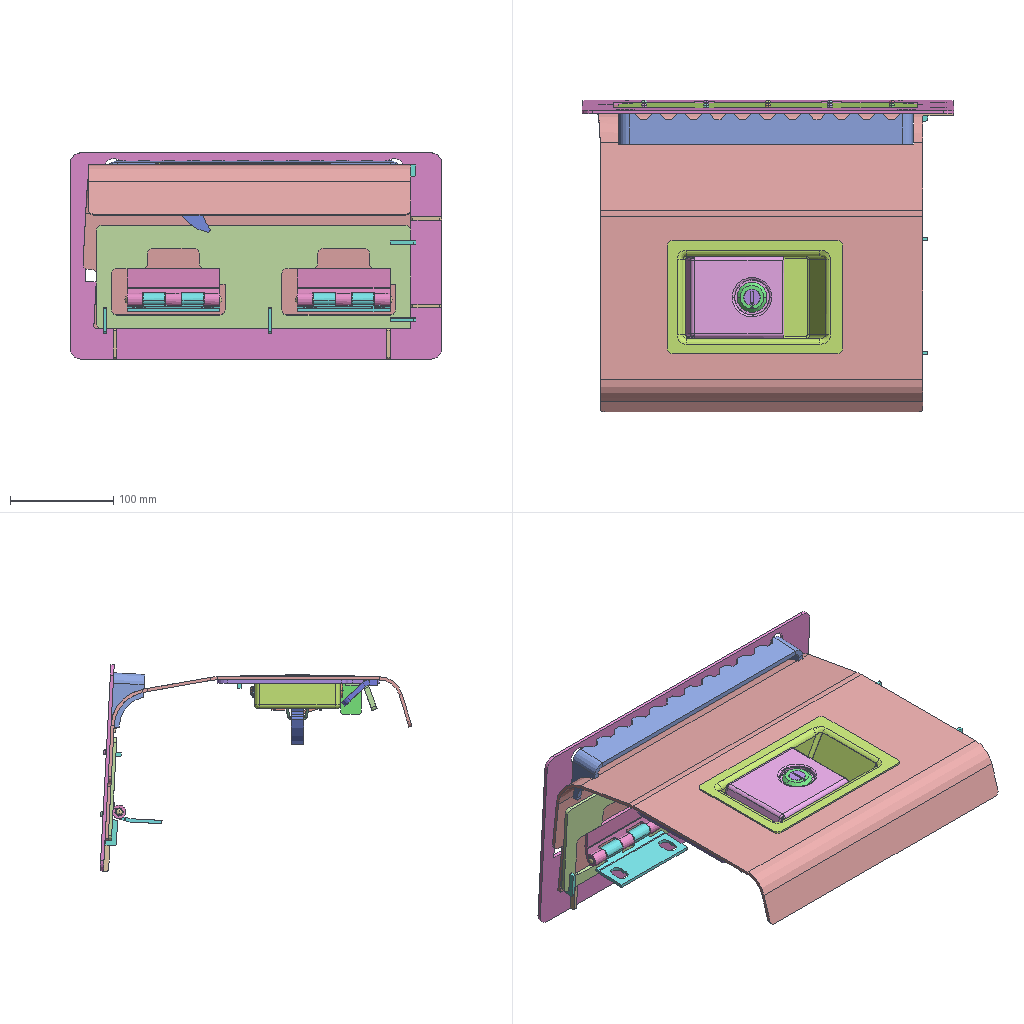Assembly | SolidWorks | 14 different items | 24 placed | box 360 x 302 x 200 mm
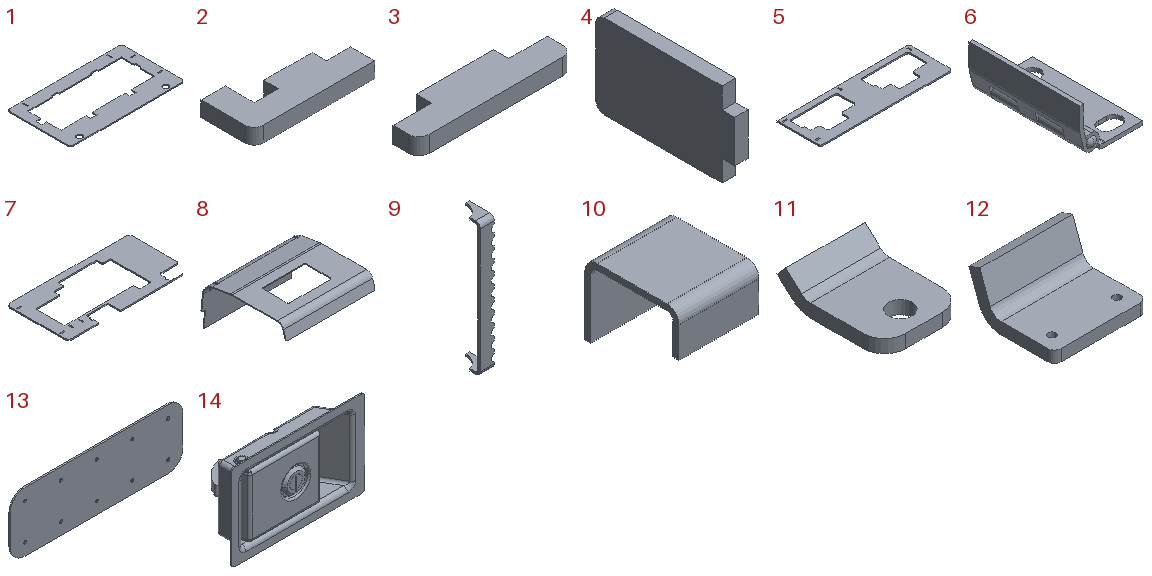Parts list (item | quantity | size | volume | features):
1 | x1 | 360 x 200 x 3.2 mm | 125012 mm3 | features FlatPattern 1, SMBaseFlange 1, SheetMetal 1
2 | x6 | 25 x 11 x 3.2 mm | 589.253 mm3 | features FlatPattern 1, SMBaseFlange 1, SheetMetal 1
3 | x4 | 30 x 8 x 3.2 mm | 618.506 mm3 | features FlatPattern 1, SMBaseFlange 1, SheetMetal 1
4 | x2 | 3.2 x 33 x 20 mm | 2011 mm3 | features FlatPattern 1, SMBaseFlange 1, SheetMetal 1
5 | x1 | 305 x 100 x 3.2 mm | 59642 mm3 | features FlatPattern 1, SMBaseFlange 1, SheetMetal 1
6 | x2 | 51.2 x 94 x 39.2 mm | 27609 mm3 | features BaseBody 3
7 | x1 | 312.3 x 157 x 3.2 mm | 83817 mm3 | features FlatPattern 1, SMBaseFlange 1, SheetMetal 1
8 | x1 | 317.63 x 297.4 x 158.457 mm | 376681 mm3 | features Fillet 2, ICE 2, FlatPattern 1, Fold 1, SMBaseFlange 1, SheetMetal 1, UnFold 1
9 | x1 | 30 x 53 x 285 mm | 47239 mm3 | features ICE 2, FlatPattern 1, SMBaseFlange 1, SheetMetal 1
10 | x1 | 40 x 47 x 36 mm | 11356 mm3 | features FlatPattern 1, SMBaseFlange 1, SheetMetal 1
11 | x1 | 30 x 40.8 x 11.858 mm | 5812 mm3 | features Fillet 1, FlatPattern 1, ICE 1, SMBaseFlange 1, SheetMetal 1
12 | x1 | 40 x 36.8 x 20.501 mm | 8922 mm3 | features Fillet 1, FlatPattern 1, HoleWzd 1, ICE 1, SMBaseFlange 1, SheetMetal 1
13 | x1 | 290 x 6 x 100 mm | 57219 mm3 | features Fillet 10, FlatPattern 1, ICE 1, SMBaseFlange 1, SheetMetal 1
14 | x1 | 170 x 67.2 x 110 mm | 99328 mm3 | features BaseBody 17
Mates (type | each side: item.copy, entity, surface, feature):
Coincident | 8.1 face plane Base-Flange1 | 9.1 face plane Base-Flange1
DistanceDim | 8.1 face plane Cut-Extrude2 | 9.1 face plane Base-Flange1
Coincident | 8.1 face plane Cut-Extrude2 | 9.1 face plane Base-Flange1
Coincident | 8.1 face plane Base-Flange1 | 13.1 face plane Base-Flange1
DistanceDim | 13.1 face plane Base-Flange1 | 8.1 face plane Base-Flange1 | 2 times
Coincident | 8.1 face plane Base-Flange1 | 10.1 edge | 2 times
DistanceDim | 8.1 face plane Cut-Extrude1 | 10.1 face cylinder Base Bend1
DistanceDim | 8.1 face plane Base-Flange1 | 10.1 face plane Base-Flange1
Coincident | 8.1 face plane Base-Flange1 | 11.1 face plane Base-Flange1
DistanceDim | 11.1 face plane Base-Flange1 | 8.1 face plane Cut-Extrude2
DistanceDim | 8.1 face plane Cut-Extrude1 | 11.1 face plane Base-Flange1
Coincident | 8.1 face plane Base-Flange1 | 12.1 face plane Base-Flange1
DistanceDim | 12.1 face plane Base-Flange1 | 8.1 face plane Base-Flange1
Coincident | 8.1 face plane Cut-Extrude1 | 12.1 face plane Base-Flange1
Coincident | 8.1 face plane Base-Flange1 | 6.1 face plane 2A6-54-11251_D90_B1_ASM.stp-1/2A6-54-11251-01_B1.stp-1-solid1
DistanceDim | 6.1 face plane 2A6-54-11251_D90_B1_ASM.stp-1/2A6-54-11251-01_B1.stp-1-solid1 | 8.1 face plane Base-Flange1 | 2 times
Coincident | 8.1 face plane Base-Flange1 | 14.1 face plane 20y-54-71491.asm.STEP-1/20y-54-71491-01.prt.STEP-1-solid1
DistanceDim | 8.1 face plane Cut-Extrude1 | 14.1 face plane 20y-54-71491.asm.STEP-1/20y-54-71491-01.prt.STEP-1-solid1
DistanceDim | 14.1 face plane 20y-54-71491.asm.STEP-1/20y-54-71491-01.prt.STEP-1-solid1 | 8.1 face plane Base-Flange1
InPlace | 8.1 face plane Base-Flange1 | 5.1 plane
InPlace | 8.1 face plane Base-Flange1 | 1.1 plane
InPlace | 2.1 plane | assembly plane
Coincident | 5.1 face plane Base-Flange1 | 2.2 face plane Base-Flange1 | 2 times
DistanceDim | 5.1 face plane Base-Flange1 | 2.2 face plane Base-Flange1
InPlace | 3.1 plane | assembly plane
Coincident | 1.1 face plane Base-Flange1 | 3.2 face plane Base-Flange1
Coincident | 8.1 face plane Base-Flange1 | 3.2 face plane Base-Flange1
DistanceDim | 3.2 face plane Base-Flange1 | 1.1 face plane Base-Flange1
InPlace | 8.1 face plane Base-Flange1 | 7.1 plane
Coincident | 7.1 face plane Base-Flange1 | 2.3 face plane Base-Flange1 | 2 times
DistanceDim | 7.1 face plane Base-Flange1 | 2.3 face plane Base-Flange1
Coincident | 7.1 face plane Base-Flange1 | 4.1 face plane Base-Flange1
Tangent | 10.1 face cylinder Base Bend1 | 4.1 face plane Base-Flange1
DistanceDim | 7.1 face plane Base-Flange1 | 4.1 face plane Base-Flange1